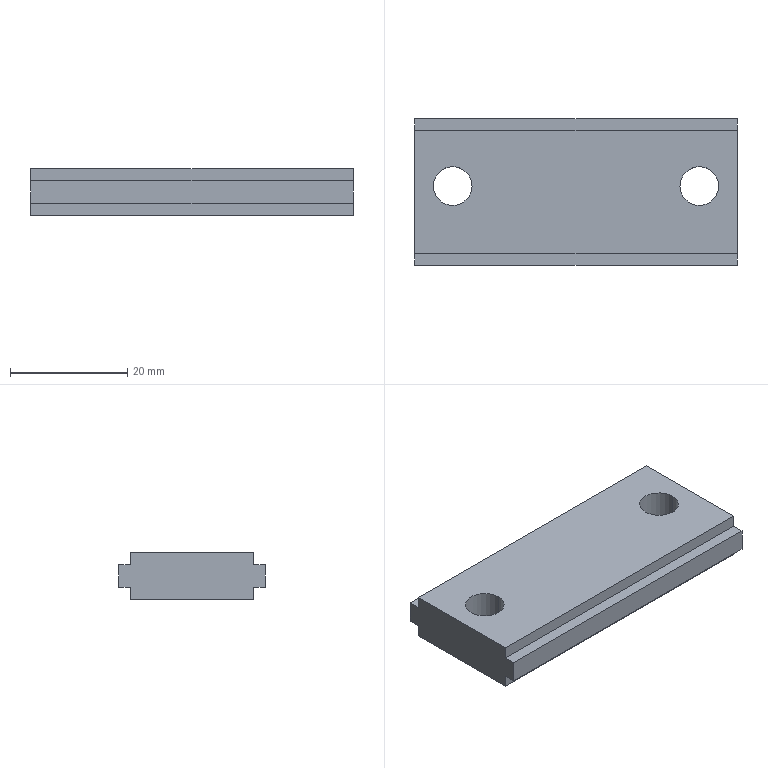Part | STEP file | 11-FG-B02811 | 1 solid | 18 faces | box 55 x 25 x 8 mm | volume 9529 mm3 | plane 14 | cylinder 4 | commonest cylinder face diameters 6.6 x4
STEP:
#1=CARTESIAN_POINT('',(51.8,13.5,0.));
#2=VERTEX_POINT('',#1);
#3=CARTESIAN_POINT('',(45.2,13.5,0.));
#4=VERTEX_POINT('',#3);
#5=CARTESIAN_POINT('',(48.5,13.5,0.));
#6=DIRECTION('',(0.,0.,-1.));
#7=DIRECTION('',(-1.,0.,0.));
#8=AXIS2_PLACEMENT_3D('',#5,#6,#7);
#9=CIRCLE('',#8,3.3);
#10=EDGE_CURVE('',#2,#4,#9,.T.);
#11=ORIENTED_EDGE('',*,*,#10,.T.);
#12=CARTESIAN_POINT('',(45.2,13.5,8.));
#13=VERTEX_POINT('',#12);
#14=CARTESIAN_POINT('',(45.2,13.5,-8.));
#15=DIRECTION('',(0.,0.,1.));
#16=VECTOR('',#15,1000.);
#17=LINE('',#14,#16);
#18=EDGE_CURVE('',#4,#13,#17,.T.);
#19=ORIENTED_EDGE('',*,*,#18,.T.);
#20=CARTESIAN_POINT('',(51.8,13.5,8.));
#21=VERTEX_POINT('',#20);
#22=CARTESIAN_POINT('',(48.5,13.5,8.));
#23=DIRECTION('',(0.,0.,1.));
#24=DIRECTION('',(1.,0.,0.));
#25=AXIS2_PLACEMENT_3D('',#22,#23,#24);
#26=CIRCLE('',#25,3.3);
#27=EDGE_CURVE('',#13,#21,#26,.T.);
#28=ORIENTED_EDGE('',*,*,#27,.T.);
#29=CARTESIAN_POINT('',(51.8,13.5,-8.));
#30=DIRECTION('',(0.,0.,1.));
#31=VECTOR('',#30,1000.);
#32=LINE('',#29,#31);
#33=EDGE_CURVE('',#2,#21,#32,.T.);
#34=ORIENTED_EDGE('',*,*,#33,.F.);
#35=EDGE_LOOP('',(#11,#19,#28,#34));
#36=FACE_OUTER_BOUND('',#35,.T.);
#37=CARTESIAN_POINT('',(48.5,13.5,-8.));
#38=DIRECTION('',(0.,0.,1.));
#39=DIRECTION('',(1.,0.,0.));
#40=AXIS2_PLACEMENT_3D('',#37,#38,#39);
#41=CYLINDRICAL_SURFACE('',#40,3.3);
#42=ADVANCED_FACE('',(#36),#41,.F.);
#43=CARTESIAN_POINT('',(9.8,13.5,0.));
#44=VERTEX_POINT('',#43);
#45=CARTESIAN_POINT('',(3.2,13.5,0.));
#46=VERTEX_POINT('',#45);
#47=CARTESIAN_POINT('',(6.5,13.5,0.));
#48=DIRECTION('',(0.,0.,-1.));
#49=DIRECTION('',(-1.,0.,0.));
#50=AXIS2_PLACEMENT_3D('',#47,#48,#49);
#51=CIRCLE('',#50,3.3);
#52=EDGE_CURVE('',#44,#46,#51,.T.);
#53=ORIENTED_EDGE('',*,*,#52,.T.);
#54=CARTESIAN_POINT('',(3.2,13.5,8.));
#55=VERTEX_POINT('',#54);
#56=CARTESIAN_POINT('',(3.2,13.5,-8.));
#57=DIRECTION('',(0.,0.,1.));
#58=VECTOR('',#57,1000.);
#59=LINE('',#56,#58);
#60=EDGE_CURVE('',#46,#55,#59,.T.);
#61=ORIENTED_EDGE('',*,*,#60,.T.);
#62=CARTESIAN_POINT('',(9.8,13.5,8.));
#63=VERTEX_POINT('',#62);
#64=CARTESIAN_POINT('',(6.5,13.5,8.));
#65=DIRECTION('',(0.,0.,1.));
#66=DIRECTION('',(1.,0.,0.));
#67=AXIS2_PLACEMENT_3D('',#64,#65,#66);
#68=CIRCLE('',#67,3.3);
#69=EDGE_CURVE('',#55,#63,#68,.T.);
#70=ORIENTED_EDGE('',*,*,#69,.T.);
#71=CARTESIAN_POINT('',(9.8,13.5,-8.));
#72=DIRECTION('',(0.,0.,1.));
#73=VECTOR('',#72,1000.);
#74=LINE('',#71,#73);
#75=EDGE_CURVE('',#44,#63,#74,.T.);
#76=ORIENTED_EDGE('',*,*,#75,.F.);
#77=EDGE_LOOP('',(#53,#61,#70,#76));
#78=FACE_OUTER_BOUND('',#77,.T.);
#79=CARTESIAN_POINT('',(6.5,13.5,-8.));
#80=DIRECTION('',(0.,0.,1.));
#81=DIRECTION('',(1.,0.,0.));
#82=AXIS2_PLACEMENT_3D('',#79,#80,#81);
#83=CYLINDRICAL_SURFACE('',#82,3.3);
#84=ADVANCED_FACE('',(#78),#83,.F.);
#85=CARTESIAN_POINT('',(0.,0.,5.9));
#86=VERTEX_POINT('',#85);
#87=CARTESIAN_POINT('',(0.,2.,5.9));
#88=VERTEX_POINT('',#87);
#89=CARTESIAN_POINT('',(0.,0.,5.9));
#90=DIRECTION('',(0.,1.,0.));
#91=VECTOR('',#90,1000.);
#92=LINE('',#89,#91);
#93=EDGE_CURVE('',#86,#88,#92,.T.);
#94=ORIENTED_EDGE('',*,*,#93,.T.);
#95=CARTESIAN_POINT('',(0.,2.,8.));
#96=VERTEX_POINT('',#95);
#97=CARTESIAN_POINT('',(0.,2.,6.));
#98=DIRECTION('',(0.,0.,1.));
#99=VECTOR('',#98,1000.);
#100=LINE('',#97,#99);
#101=EDGE_CURVE('',#88,#96,#100,.T.);
#102=ORIENTED_EDGE('',*,*,#101,.T.);
#103=CARTESIAN_POINT('',(0.,23.,8.));
#104=VERTEX_POINT('',#103);
#105=CARTESIAN_POINT('',(0.,2.,8.));
#106=DIRECTION('',(0.,1.,0.));
#107=VECTOR('',#106,1000.);
#108=LINE('',#105,#107);
#109=EDGE_CURVE('',#96,#104,#108,.T.);
#110=ORIENTED_EDGE('',*,*,#109,.T.);
#111=CARTESIAN_POINT('',(0.,23.,5.9));
#112=VERTEX_POINT('',#111);
#113=CARTESIAN_POINT('',(0.,23.,6.));
#114=DIRECTION('',(0.,0.,-1.));
#115=VECTOR('',#114,1000.);
#116=LINE('',#113,#115);
#117=EDGE_CURVE('',#104,#112,#116,.T.);
#118=ORIENTED_EDGE('',*,*,#117,.T.);
#119=CARTESIAN_POINT('',(0.,25.,5.9));
#120=VERTEX_POINT('',#119);
#121=CARTESIAN_POINT('',(0.,0.,5.9));
#122=DIRECTION('',(0.,1.,0.));
#123=VECTOR('',#122,1000.);
#124=LINE('',#121,#123);
#125=EDGE_CURVE('',#112,#120,#124,.T.);
#126=ORIENTED_EDGE('',*,*,#125,.T.);
#127=CARTESIAN_POINT('',(0.,25.,2.1));
#128=VERTEX_POINT('',#127);
#129=CARTESIAN_POINT('',(0.,25.,6.));
#130=DIRECTION('',(0.,0.,-1.));
#131=VECTOR('',#130,1000.);
#132=LINE('',#129,#131);
#133=EDGE_CURVE('',#120,#128,#132,.T.);
#134=ORIENTED_EDGE('',*,*,#133,.T.);
#135=CARTESIAN_POINT('',(0.,23.,2.1));
#136=VERTEX_POINT('',#135);
#137=CARTESIAN_POINT('',(0.,0.,2.1));
#138=DIRECTION('',(0.,-1.,0.));
#139=VECTOR('',#138,1000.);
#140=LINE('',#137,#139);
#141=EDGE_CURVE('',#128,#136,#140,.T.);
#142=ORIENTED_EDGE('',*,*,#141,.T.);
#143=CARTESIAN_POINT('',(0.,23.,0.));
#144=VERTEX_POINT('',#143);
#145=CARTESIAN_POINT('',(0.,23.,6.));
#146=DIRECTION('',(0.,0.,-1.));
#147=VECTOR('',#146,1000.);
#148=LINE('',#145,#147);
#149=EDGE_CURVE('',#136,#144,#148,.T.);
#150=ORIENTED_EDGE('',*,*,#149,.T.);
#151=CARTESIAN_POINT('',(0.,2.,0.));
#152=VERTEX_POINT('',#151);
#153=CARTESIAN_POINT('',(0.,0.,0.));
#154=DIRECTION('',(0.,-1.,0.));
#155=VECTOR('',#154,1000.);
#156=LINE('',#153,#155);
#157=EDGE_CURVE('',#144,#152,#156,.T.);
#158=ORIENTED_EDGE('',*,*,#157,.T.);
#159=CARTESIAN_POINT('',(0.,2.,2.1));
#160=VERTEX_POINT('',#159);
#161=CARTESIAN_POINT('',(0.,2.,6.));
#162=DIRECTION('',(0.,0.,1.));
#163=VECTOR('',#162,1000.);
#164=LINE('',#161,#163);
#165=EDGE_CURVE('',#152,#160,#164,.T.);
#166=ORIENTED_EDGE('',*,*,#165,.T.);
#167=CARTESIAN_POINT('',(0.,0.,2.1));
#168=VERTEX_POINT('',#167);
#169=CARTESIAN_POINT('',(0.,0.,2.1));
#170=DIRECTION('',(0.,-1.,0.));
#171=VECTOR('',#170,1000.);
#172=LINE('',#169,#171);
#173=EDGE_CURVE('',#160,#168,#172,.T.);
#174=ORIENTED_EDGE('',*,*,#173,.T.);
#175=CARTESIAN_POINT('',(0.,0.,6.));
#176=DIRECTION('',(0.,0.,-1.));
#177=VECTOR('',#176,1000.);
#178=LINE('',#175,#177);
#179=EDGE_CURVE('',#86,#168,#178,.T.);
#180=ORIENTED_EDGE('',*,*,#179,.F.);
#181=EDGE_LOOP('',(#94,#102,#110,#118,#126,#134,#142,#150,#158,#166,#174,#180));
#182=FACE_OUTER_BOUND('',#181,.T.);
#183=CARTESIAN_POINT('',(0.,0.,6.));
#184=DIRECTION('',(1.,0.,0.));
#185=DIRECTION('',(0.,1.,0.));
#186=AXIS2_PLACEMENT_3D('',#183,#184,#185);
#187=PLANE('',#186);
#188=ADVANCED_FACE('',(#182),#187,.F.);
#189=CARTESIAN_POINT('',(55.,0.,5.9));
#190=VERTEX_POINT('',#189);
#191=CARTESIAN_POINT('',(55.,0.,2.1));
#192=VERTEX_POINT('',#191);
#193=CARTESIAN_POINT('',(55.,0.,6.));
#194=DIRECTION('',(0.,0.,-1.));
#195=VECTOR('',#194,1000.);
#196=LINE('',#193,#195);
#197=EDGE_CURVE('',#190,#192,#196,.T.);
#198=ORIENTED_EDGE('',*,*,#197,.F.);
#199=CARTESIAN_POINT('',(-9.,0.,5.9));
#200=DIRECTION('',(1.,0.,0.));
#201=VECTOR('',#200,1000.);
#202=LINE('',#199,#201);
#203=EDGE_CURVE('',#86,#190,#202,.T.);
#204=ORIENTED_EDGE('',*,*,#203,.F.);
#205=ORIENTED_EDGE('',*,*,#179,.T.);
#206=CARTESIAN_POINT('',(-52.,0.,2.1));
#207=DIRECTION('',(1.,0.,0.));
#208=VECTOR('',#207,1000.);
#209=LINE('',#206,#208);
#210=EDGE_CURVE('',#168,#192,#209,.T.);
#211=ORIENTED_EDGE('',*,*,#210,.T.);
#212=EDGE_LOOP('',(#198,#204,#205,#211));
#213=FACE_OUTER_BOUND('',#212,.T.);
#214=CARTESIAN_POINT('',(0.,0.,6.));
#215=DIRECTION('',(0.,1.,0.));
#216=DIRECTION('',(0.,0.,1.));
#217=AXIS2_PLACEMENT_3D('',#214,#215,#216);
#218=PLANE('',#217);
#219=ADVANCED_FACE('',(#213),#218,.F.);
#220=CARTESIAN_POINT('',(55.,2.,8.));
#221=VERTEX_POINT('',#220);
#222=CARTESIAN_POINT('',(55.,2.,5.9));
#223=VERTEX_POINT('',#222);
#224=CARTESIAN_POINT('',(55.,2.,6.));
#225=DIRECTION('',(0.,0.,-1.));
#226=VECTOR('',#225,1000.);
#227=LINE('',#224,#226);
#228=EDGE_CURVE('',#221,#223,#227,.T.);
#229=ORIENTED_EDGE('',*,*,#228,.T.);
#230=CARTESIAN_POINT('',(55.,2.,5.9));
#231=DIRECTION('',(0.,1.,0.));
#232=VECTOR('',#231,1000.);
#233=LINE('',#230,#232);
#234=EDGE_CURVE('',#190,#223,#233,.T.);
#235=ORIENTED_EDGE('',*,*,#234,.F.);
#236=ORIENTED_EDGE('',*,*,#197,.T.);
#237=CARTESIAN_POINT('',(55.,2.,2.1));
#238=VERTEX_POINT('',#237);
#239=CARTESIAN_POINT('',(55.,0.,2.1));
#240=DIRECTION('',(0.,-1.,0.));
#241=VECTOR('',#240,1000.);
#242=LINE('',#239,#241);
#243=EDGE_CURVE('',#238,#192,#242,.T.);
#244=ORIENTED_EDGE('',*,*,#243,.F.);
#245=CARTESIAN_POINT('',(55.,2.,0.));
#246=VERTEX_POINT('',#245);
#247=CARTESIAN_POINT('',(55.,2.,0.));
#248=DIRECTION('',(0.,0.,1.));
#249=VECTOR('',#248,1000.);
#250=LINE('',#247,#249);
#251=EDGE_CURVE('',#246,#238,#250,.T.);
#252=ORIENTED_EDGE('',*,*,#251,.F.);
#253=CARTESIAN_POINT('',(55.,23.,0.));
#254=VERTEX_POINT('',#253);
#255=CARTESIAN_POINT('',(55.,0.,0.));
#256=DIRECTION('',(0.,1.,0.));
#257=VECTOR('',#256,1000.);
#258=LINE('',#255,#257);
#259=EDGE_CURVE('',#246,#254,#258,.T.);
#260=ORIENTED_EDGE('',*,*,#259,.T.);
#261=CARTESIAN_POINT('',(55.,23.,2.1));
#262=VERTEX_POINT('',#261);
#263=CARTESIAN_POINT('',(55.,23.,0.));
#264=DIRECTION('',(0.,0.,-1.));
#265=VECTOR('',#264,1000.);
#266=LINE('',#263,#265);
#267=EDGE_CURVE('',#262,#254,#266,.T.);
#268=ORIENTED_EDGE('',*,*,#267,.F.);
#269=CARTESIAN_POINT('',(55.,25.,2.1));
#270=VERTEX_POINT('',#269);
#271=CARTESIAN_POINT('',(55.,25.,2.1));
#272=DIRECTION('',(0.,-1.,0.));
#273=VECTOR('',#272,1000.);
#274=LINE('',#271,#273);
#275=EDGE_CURVE('',#270,#262,#274,.T.);
#276=ORIENTED_EDGE('',*,*,#275,.F.);
#277=CARTESIAN_POINT('',(55.,25.,5.9));
#278=VERTEX_POINT('',#277);
#279=CARTESIAN_POINT('',(55.,25.,6.));
#280=DIRECTION('',(0.,0.,-1.));
#281=VECTOR('',#280,1000.);
#282=LINE('',#279,#281);
#283=EDGE_CURVE('',#278,#270,#282,.T.);
#284=ORIENTED_EDGE('',*,*,#283,.F.);
#285=CARTESIAN_POINT('',(55.,23.,5.9));
#286=VERTEX_POINT('',#285);
#287=CARTESIAN_POINT('',(55.,23.,5.9));
#288=DIRECTION('',(0.,1.,0.));
#289=VECTOR('',#288,1000.);
#290=LINE('',#287,#289);
#291=EDGE_CURVE('',#286,#278,#290,.T.);
#292=ORIENTED_EDGE('',*,*,#291,.F.);
#293=CARTESIAN_POINT('',(55.,23.,8.));
#294=VERTEX_POINT('',#293);
#295=CARTESIAN_POINT('',(55.,23.,6.));
#296=DIRECTION('',(0.,0.,1.));
#297=VECTOR('',#296,1000.);
#298=LINE('',#295,#297);
#299=EDGE_CURVE('',#286,#294,#298,.T.);
#300=ORIENTED_EDGE('',*,*,#299,.T.);
#301=CARTESIAN_POINT('',(55.,2.,8.));
#302=DIRECTION('',(0.,-1.,0.));
#303=VECTOR('',#302,1000.);
#304=LINE('',#301,#303);
#305=EDGE_CURVE('',#294,#221,#304,.T.);
#306=ORIENTED_EDGE('',*,*,#305,.T.);
#307=EDGE_LOOP('',(#229,#235,#236,#244,#252,#260,#268,#276,#284,#292,#300,#306));
#308=FACE_OUTER_BOUND('',#307,.T.);
#309=CARTESIAN_POINT('',(55.,0.,6.));
#310=DIRECTION('',(-1.,0.,0.));
#311=DIRECTION('',(0.,-1.,0.));
#312=AXIS2_PLACEMENT_3D('',#309,#310,#311);
#313=PLANE('',#312);
#314=ADVANCED_FACE('',(#308),#313,.F.);
#315=ORIENTED_EDGE('',*,*,#133,.F.);
#316=CARTESIAN_POINT('',(-9.,25.,5.9));
#317=DIRECTION('',(1.,0.,0.));
#318=VECTOR('',#317,1000.);
#319=LINE('',#316,#318);
#320=EDGE_CURVE('',#120,#278,#319,.T.);
#321=ORIENTED_EDGE('',*,*,#320,.T.);
#322=ORIENTED_EDGE('',*,*,#283,.T.);
#323=CARTESIAN_POINT('',(-52.,25.,2.1));
#324=DIRECTION('',(1.,0.,0.));
#325=VECTOR('',#324,1000.);
#326=LINE('',#323,#325);
#327=EDGE_CURVE('',#128,#270,#326,.T.);
#328=ORIENTED_EDGE('',*,*,#327,.F.);
#329=EDGE_LOOP('',(#315,#321,#322,#328));
#330=FACE_OUTER_BOUND('',#329,.T.);
#331=CARTESIAN_POINT('',(0.,25.,6.));
#332=DIRECTION('',(0.,-1.,0.));
#333=DIRECTION('',(0.,0.,-1.));
#334=AXIS2_PLACEMENT_3D('',#331,#332,#333);
#335=PLANE('',#334);
#336=ADVANCED_FACE('',(#330),#335,.F.);
#337=ORIENTED_EDGE('',*,*,#10,.F.);
#338=CARTESIAN_POINT('',(48.5,13.5,0.));
#339=DIRECTION('',(0.,0.,-1.));
#340=DIRECTION('',(-1.,0.,0.));
#341=AXIS2_PLACEMENT_3D('',#338,#339,#340);
#342=CIRCLE('',#341,3.3);
#343=EDGE_CURVE('',#4,#2,#342,.T.);
#344=ORIENTED_EDGE('',*,*,#343,.F.);
#345=EDGE_LOOP('',(#337,#344));
#346=FACE_BOUND('',#345,.T.);
#347=ORIENTED_EDGE('',*,*,#52,.F.);
#348=CARTESIAN_POINT('',(6.5,13.5,0.));
#349=DIRECTION('',(0.,0.,-1.));
#350=DIRECTION('',(-1.,0.,0.));
#351=AXIS2_PLACEMENT_3D('',#348,#349,#350);
#352=CIRCLE('',#351,3.3);
#353=EDGE_CURVE('',#46,#44,#352,.T.);
#354=ORIENTED_EDGE('',*,*,#353,.F.);
#355=EDGE_LOOP('',(#347,#354));
#356=FACE_BOUND('',#355,.T.);
#357=CARTESIAN_POINT('',(0.,23.,0.));
#358=DIRECTION('',(-1.,0.,0.));
#359=VECTOR('',#358,1000.);
#360=LINE('',#357,#359);
#361=EDGE_CURVE('',#254,#144,#360,.T.);
#362=ORIENTED_EDGE('',*,*,#361,.F.);
#363=ORIENTED_EDGE('',*,*,#259,.F.);
#364=CARTESIAN_POINT('',(0.,2.,0.));
#365=DIRECTION('',(1.,0.,0.));
#366=VECTOR('',#365,1000.);
#367=LINE('',#364,#366);
#368=EDGE_CURVE('',#152,#246,#367,.T.);
#369=ORIENTED_EDGE('',*,*,#368,.F.);
#370=ORIENTED_EDGE('',*,*,#157,.F.);
#371=EDGE_LOOP('',(#362,#363,#369,#370));
#372=FACE_OUTER_BOUND('',#371,.T.);
#373=CARTESIAN_POINT('',(0.,25.,0.));
#374=DIRECTION('',(0.,0.,-1.));
#375=DIRECTION('',(-1.,0.,0.));
#376=AXIS2_PLACEMENT_3D('',#373,#374,#375);
#377=PLANE('',#376);
#378=ADVANCED_FACE('',(#346,#356,#372),#377,.T.);
#379=CARTESIAN_POINT('',(-52.,2.,2.1));
#380=DIRECTION('',(1.,0.,0.));
#381=VECTOR('',#380,1000.);
#382=LINE('',#379,#381);
#383=EDGE_CURVE('',#160,#238,#382,.T.);
#384=ORIENTED_EDGE('',*,*,#383,.T.);
#385=ORIENTED_EDGE('',*,*,#243,.T.);
#386=ORIENTED_EDGE('',*,*,#210,.F.);
#387=ORIENTED_EDGE('',*,*,#173,.F.);
#388=EDGE_LOOP('',(#384,#385,#386,#387));
#389=FACE_OUTER_BOUND('',#388,.T.);
#390=CARTESIAN_POINT('',(-52.,0.,2.1));
#391=DIRECTION('',(0.,0.,1.));
#392=DIRECTION('',(1.,0.,0.));
#393=AXIS2_PLACEMENT_3D('',#390,#391,#392);
#394=PLANE('',#393);
#395=ADVANCED_FACE('',(#389),#394,.F.);
#396=ORIENTED_EDGE('',*,*,#368,.T.);
#397=ORIENTED_EDGE('',*,*,#251,.T.);
#398=ORIENTED_EDGE('',*,*,#383,.F.);
#399=ORIENTED_EDGE('',*,*,#165,.F.);
#400=EDGE_LOOP('',(#396,#397,#398,#399));
#401=FACE_OUTER_BOUND('',#400,.T.);
#402=CARTESIAN_POINT('',(-52.,2.,0.));
#403=DIRECTION('',(0.,1.,0.));
#404=DIRECTION('',(0.,0.,1.));
#405=AXIS2_PLACEMENT_3D('',#402,#403,#404);
#406=PLANE('',#405);
#407=ADVANCED_FACE('',(#401),#406,.F.);
#408=ORIENTED_EDGE('',*,*,#327,.T.);
#409=ORIENTED_EDGE('',*,*,#275,.T.);
#410=CARTESIAN_POINT('',(-52.,23.,2.1));
#411=DIRECTION('',(1.,0.,0.));
#412=VECTOR('',#411,1000.);
#413=LINE('',#410,#412);
#414=EDGE_CURVE('',#136,#262,#413,.T.);
#415=ORIENTED_EDGE('',*,*,#414,.F.);
#416=ORIENTED_EDGE('',*,*,#141,.F.);
#417=EDGE_LOOP('',(#408,#409,#415,#416));
#418=FACE_OUTER_BOUND('',#417,.T.);
#419=CARTESIAN_POINT('',(-52.,25.,2.1));
#420=DIRECTION('',(0.,0.,1.));
#421=DIRECTION('',(0.,-1.,0.));
#422=AXIS2_PLACEMENT_3D('',#419,#420,#421);
#423=PLANE('',#422);
#424=ADVANCED_FACE('',(#418),#423,.F.);
#425=ORIENTED_EDGE('',*,*,#414,.T.);
#426=ORIENTED_EDGE('',*,*,#267,.T.);
#427=ORIENTED_EDGE('',*,*,#361,.T.);
#428=ORIENTED_EDGE('',*,*,#149,.F.);
#429=EDGE_LOOP('',(#425,#426,#427,#428));
#430=FACE_OUTER_BOUND('',#429,.T.);
#431=CARTESIAN_POINT('',(-52.,23.,0.));
#432=DIRECTION('',(0.,-1.,0.));
#433=DIRECTION('',(0.,0.,-1.));
#434=AXIS2_PLACEMENT_3D('',#431,#432,#433);
#435=PLANE('',#434);
#436=ADVANCED_FACE('',(#430),#435,.F.);
#437=ORIENTED_EDGE('',*,*,#101,.F.);
#438=CARTESIAN_POINT('',(-9.,2.,5.9));
#439=DIRECTION('',(1.,0.,0.));
#440=VECTOR('',#439,1000.);
#441=LINE('',#438,#440);
#442=EDGE_CURVE('',#88,#223,#441,.T.);
#443=ORIENTED_EDGE('',*,*,#442,.T.);
#444=ORIENTED_EDGE('',*,*,#228,.F.);
#445=CARTESIAN_POINT('',(-21.095,2.,8.));
#446=DIRECTION('',(1.,0.,0.));
#447=VECTOR('',#446,1000.);
#448=LINE('',#445,#447);
#449=EDGE_CURVE('',#96,#221,#448,.T.);
#450=ORIENTED_EDGE('',*,*,#449,.F.);
#451=EDGE_LOOP('',(#437,#443,#444,#450));
#452=FACE_OUTER_BOUND('',#451,.T.);
#453=CARTESIAN_POINT('',(-21.095,2.,6.));
#454=DIRECTION('',(0.,-1.,0.));
#455=DIRECTION('',(0.,0.,-1.));
#456=AXIS2_PLACEMENT_3D('',#453,#454,#455);
#457=PLANE('',#456);
#458=ADVANCED_FACE('',(#452),#457,.T.);
#459=CARTESIAN_POINT('',(48.5,13.5,8.));
#460=DIRECTION('',(0.,0.,1.));
#461=DIRECTION('',(1.,0.,0.));
#462=AXIS2_PLACEMENT_3D('',#459,#460,#461);
#463=CIRCLE('',#462,3.3);
#464=EDGE_CURVE('',#21,#13,#463,.T.);
#465=ORIENTED_EDGE('',*,*,#464,.F.);
#466=ORIENTED_EDGE('',*,*,#27,.F.);
#467=EDGE_LOOP('',(#465,#466));
#468=FACE_BOUND('',#467,.T.);
#469=CARTESIAN_POINT('',(6.5,13.5,8.));
#470=DIRECTION('',(0.,0.,1.));
#471=DIRECTION('',(1.,0.,0.));
#472=AXIS2_PLACEMENT_3D('',#469,#470,#471);
#473=CIRCLE('',#472,3.3);
#474=EDGE_CURVE('',#63,#55,#473,.T.);
#475=ORIENTED_EDGE('',*,*,#474,.F.);
#476=ORIENTED_EDGE('',*,*,#69,.F.);
#477=EDGE_LOOP('',(#475,#476));
#478=FACE_BOUND('',#477,.T.);
#479=ORIENTED_EDGE('',*,*,#109,.F.);
#480=ORIENTED_EDGE('',*,*,#449,.T.);
#481=ORIENTED_EDGE('',*,*,#305,.F.);
#482=CARTESIAN_POINT('',(-21.095,23.,8.));
#483=DIRECTION('',(1.,0.,0.));
#484=VECTOR('',#483,1000.);
#485=LINE('',#482,#484);
#486=EDGE_CURVE('',#104,#294,#485,.T.);
#487=ORIENTED_EDGE('',*,*,#486,.F.);
#488=EDGE_LOOP('',(#479,#480,#481,#487));
#489=FACE_OUTER_BOUND('',#488,.T.);
#490=CARTESIAN_POINT('',(-21.095,2.,8.));
#491=DIRECTION('',(0.,0.,1.));
#492=DIRECTION('',(1.,0.,0.));
#493=AXIS2_PLACEMENT_3D('',#490,#491,#492);
#494=PLANE('',#493);
#495=ADVANCED_FACE('',(#468,#478,#489),#494,.T.);
#496=ORIENTED_EDGE('',*,*,#117,.F.);
#497=ORIENTED_EDGE('',*,*,#486,.T.);
#498=ORIENTED_EDGE('',*,*,#299,.F.);
#499=CARTESIAN_POINT('',(-9.,23.,5.9));
#500=DIRECTION('',(1.,0.,0.));
#501=VECTOR('',#500,1000.);
#502=LINE('',#499,#501);
#503=EDGE_CURVE('',#112,#286,#502,.T.);
#504=ORIENTED_EDGE('',*,*,#503,.F.);
#505=EDGE_LOOP('',(#496,#497,#498,#504));
#506=FACE_OUTER_BOUND('',#505,.T.);
#507=CARTESIAN_POINT('',(-21.095,23.,6.));
#508=DIRECTION('',(0.,1.,0.));
#509=DIRECTION('',(0.,0.,1.));
#510=AXIS2_PLACEMENT_3D('',#507,#508,#509);
#511=PLANE('',#510);
#512=ADVANCED_FACE('',(#506),#511,.T.);
#513=ORIENTED_EDGE('',*,*,#60,.F.);
#514=ORIENTED_EDGE('',*,*,#353,.T.);
#515=ORIENTED_EDGE('',*,*,#75,.T.);
#516=ORIENTED_EDGE('',*,*,#474,.T.);
#517=EDGE_LOOP('',(#513,#514,#515,#516));
#518=FACE_OUTER_BOUND('',#517,.T.);
#519=CARTESIAN_POINT('',(6.5,13.5,-8.));
#520=DIRECTION('',(0.,0.,1.));
#521=DIRECTION('',(1.,0.,0.));
#522=AXIS2_PLACEMENT_3D('',#519,#520,#521);
#523=CYLINDRICAL_SURFACE('',#522,3.3);
#524=ADVANCED_FACE('',(#518),#523,.F.);
#525=ORIENTED_EDGE('',*,*,#18,.F.);
#526=ORIENTED_EDGE('',*,*,#343,.T.);
#527=ORIENTED_EDGE('',*,*,#33,.T.);
#528=ORIENTED_EDGE('',*,*,#464,.T.);
#529=EDGE_LOOP('',(#525,#526,#527,#528));
#530=FACE_OUTER_BOUND('',#529,.T.);
#531=CARTESIAN_POINT('',(48.5,13.5,-8.));
#532=DIRECTION('',(0.,0.,1.));
#533=DIRECTION('',(1.,0.,0.));
#534=AXIS2_PLACEMENT_3D('',#531,#532,#533);
#535=CYLINDRICAL_SURFACE('',#534,3.3);
#536=ADVANCED_FACE('',(#530),#535,.F.);
#537=ORIENTED_EDGE('',*,*,#503,.T.);
#538=ORIENTED_EDGE('',*,*,#291,.T.);
#539=ORIENTED_EDGE('',*,*,#320,.F.);
#540=ORIENTED_EDGE('',*,*,#125,.F.);
#541=EDGE_LOOP('',(#537,#538,#539,#540));
#542=FACE_OUTER_BOUND('',#541,.T.);
#543=CARTESIAN_POINT('',(-9.,23.,5.9));
#544=DIRECTION('',(0.,0.,-1.));
#545=DIRECTION('',(-1.,0.,0.));
#546=AXIS2_PLACEMENT_3D('',#543,#544,#545);
#547=PLANE('',#546);
#548=ADVANCED_FACE('',(#542),#547,.F.);
#549=ORIENTED_EDGE('',*,*,#203,.T.);
#550=ORIENTED_EDGE('',*,*,#234,.T.);
#551=ORIENTED_EDGE('',*,*,#442,.F.);
#552=ORIENTED_EDGE('',*,*,#93,.F.);
#553=EDGE_LOOP('',(#549,#550,#551,#552));
#554=FACE_OUTER_BOUND('',#553,.T.);
#555=CARTESIAN_POINT('',(-9.,2.,5.9));
#556=DIRECTION('',(0.,0.,-1.));
#557=DIRECTION('',(-1.,0.,0.));
#558=AXIS2_PLACEMENT_3D('',#555,#556,#557);
#559=PLANE('',#558);
#560=ADVANCED_FACE('',(#554),#559,.F.);
#561=CLOSED_SHELL('',(#42,#84,#188,#219,#314,#336,#378,#395,#407,#424,#436,#458,#495,#512,#524,#536,#548,#560));
#562=MANIFOLD_SOLID_BREP('',#561);
#563=CARTESIAN_POINT('',(0.,0.,0.));
#564=DIRECTION('',(0.,0.,1.));
#565=DIRECTION('',(1.,0.,0.));
#566=AXIS2_PLACEMENT_3D('',#563,#564,#565);
#567=(LENGTH_UNIT()NAMED_UNIT(*)SI_UNIT(.MILLI.,.METRE.));
#568=UNCERTAINTY_MEASURE_WITH_UNIT(LENGTH_MEASURE(0.00001),#567,'','');
#569=(NAMED_UNIT(*)PLANE_ANGLE_UNIT()SI_UNIT($,.RADIAN.));
#570=(NAMED_UNIT(*)SI_UNIT($,.STERADIAN.)SOLID_ANGLE_UNIT());
#571=(GEOMETRIC_REPRESENTATION_CONTEXT(3)GLOBAL_UNCERTAINTY_ASSIGNED_CONTEXT((#568))GLOBAL_UNIT_ASSIGNED_CONTEXT((#567,#569,#570))REPRESENTATION_CONTEXT('',''));
#572=ADVANCED_BREP_SHAPE_REPRESENTATION('',(#562,#566),#571);